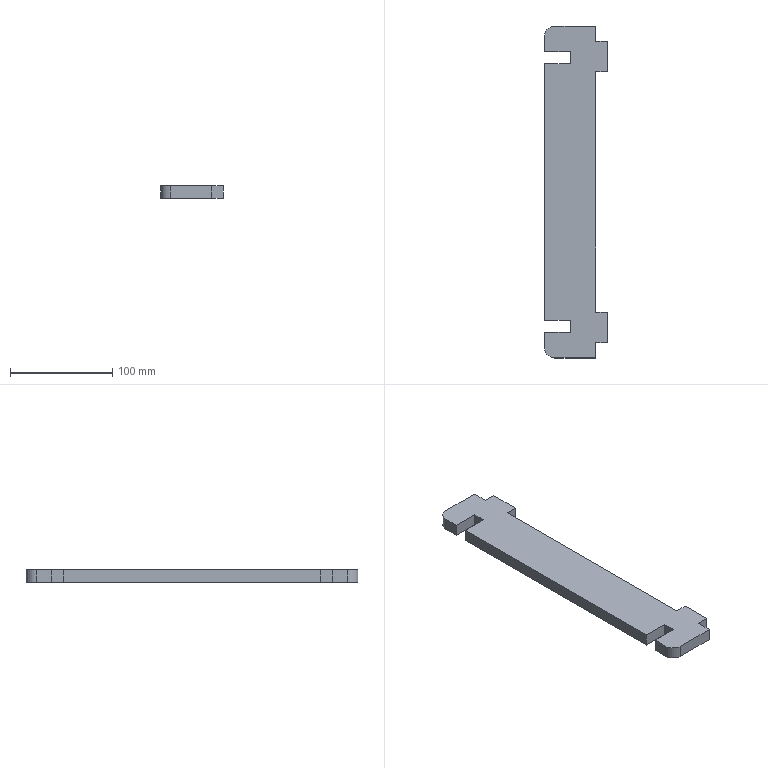Part | SolidWorks | features FlatPattern 1, SMBaseFlange 1, SheetMetal 1 | 1 solid | 24 faces | box 61.5 x 325 x 12 mm | volume 195507 mm3 | plane 22 | cylinder 2 | commonest cylinder face diameters 20 x2
STEP:
#1=CARTESIAN_POINT('',(154.972,127.382,0.));
#2=VERTEX_POINT('',#1);
#3=CARTESIAN_POINT('',(154.972,142.382,0.));
#4=VERTEX_POINT('',#3);
#5=CARTESIAN_POINT('',(154.972,142.382,0.));
#6=DIRECTION('',(0.,1.,0.));
#7=VECTOR('',#6,1000.);
#8=LINE('',#5,#7);
#9=EDGE_CURVE('',#2,#4,#8,.T.);
#10=ORIENTED_EDGE('',*,*,#9,.F.);
#11=CARTESIAN_POINT('',(154.972,127.382,-12.));
#12=VERTEX_POINT('',#11);
#13=CARTESIAN_POINT('',(154.972,127.382,-12.));
#14=DIRECTION('',(0.,0.,1.));
#15=VECTOR('',#14,1000.);
#16=LINE('',#13,#15);
#17=EDGE_CURVE('',#12,#2,#16,.T.);
#18=ORIENTED_EDGE('',*,*,#17,.F.);
#19=CARTESIAN_POINT('',(154.972,142.382,-12.));
#20=VERTEX_POINT('',#19);
#21=CARTESIAN_POINT('',(154.972,142.382,-12.));
#22=DIRECTION('',(0.,1.,0.));
#23=VECTOR('',#22,1000.);
#24=LINE('',#21,#23);
#25=EDGE_CURVE('',#12,#20,#24,.T.);
#26=ORIENTED_EDGE('',*,*,#25,.T.);
#27=CARTESIAN_POINT('',(154.972,142.382,-12.));
#28=DIRECTION('',(0.,0.,1.));
#29=VECTOR('',#28,1000.);
#30=LINE('',#27,#29);
#31=EDGE_CURVE('',#20,#4,#30,.T.);
#32=ORIENTED_EDGE('',*,*,#31,.T.);
#33=EDGE_LOOP('',(#10,#18,#26,#32));
#34=FACE_OUTER_BOUND('',#33,.T.);
#35=CARTESIAN_POINT('',(154.972,142.382,-12.));
#36=DIRECTION('',(1.,0.,0.));
#37=DIRECTION('',(0.,0.,-1.));
#38=AXIS2_PLACEMENT_3D('',#35,#36,#37);
#39=PLANE('',#38);
#40=ADVANCED_FACE('',(#34),#39,.T.);
#41=CARTESIAN_POINT('',(166.472,127.382,0.));
#42=VERTEX_POINT('',#41);
#43=CARTESIAN_POINT('',(154.972,127.382,0.));
#44=DIRECTION('',(-1.,0.,0.));
#45=VECTOR('',#44,1000.);
#46=LINE('',#43,#45);
#47=EDGE_CURVE('',#42,#2,#46,.T.);
#48=ORIENTED_EDGE('',*,*,#47,.F.);
#49=CARTESIAN_POINT('',(166.472,127.382,-12.));
#50=VERTEX_POINT('',#49);
#51=CARTESIAN_POINT('',(166.472,127.382,-12.));
#52=DIRECTION('',(0.,0.,1.));
#53=VECTOR('',#52,1000.);
#54=LINE('',#51,#53);
#55=EDGE_CURVE('',#50,#42,#54,.T.);
#56=ORIENTED_EDGE('',*,*,#55,.F.);
#57=CARTESIAN_POINT('',(154.972,127.382,-12.));
#58=DIRECTION('',(-1.,0.,0.));
#59=VECTOR('',#58,1000.);
#60=LINE('',#57,#59);
#61=EDGE_CURVE('',#50,#12,#60,.T.);
#62=ORIENTED_EDGE('',*,*,#61,.T.);
#63=ORIENTED_EDGE('',*,*,#17,.T.);
#64=EDGE_LOOP('',(#48,#56,#62,#63));
#65=FACE_OUTER_BOUND('',#64,.T.);
#66=CARTESIAN_POINT('',(154.972,127.382,-12.));
#67=DIRECTION('',(0.,1.,0.));
#68=DIRECTION('',(0.,0.,1.));
#69=AXIS2_PLACEMENT_3D('',#66,#67,#68);
#70=PLANE('',#69);
#71=ADVANCED_FACE('',(#65),#70,.T.);
#72=CARTESIAN_POINT('',(166.472,97.382,0.));
#73=VERTEX_POINT('',#72);
#74=CARTESIAN_POINT('',(166.472,127.382,0.));
#75=DIRECTION('',(0.,1.,0.));
#76=VECTOR('',#75,1000.);
#77=LINE('',#74,#76);
#78=EDGE_CURVE('',#73,#42,#77,.T.);
#79=ORIENTED_EDGE('',*,*,#78,.F.);
#80=CARTESIAN_POINT('',(166.472,97.382,-12.));
#81=VERTEX_POINT('',#80);
#82=CARTESIAN_POINT('',(166.472,97.382,-12.));
#83=DIRECTION('',(0.,0.,1.));
#84=VECTOR('',#83,1000.);
#85=LINE('',#82,#84);
#86=EDGE_CURVE('',#81,#73,#85,.T.);
#87=ORIENTED_EDGE('',*,*,#86,.F.);
#88=CARTESIAN_POINT('',(166.472,127.382,-12.));
#89=DIRECTION('',(0.,1.,0.));
#90=VECTOR('',#89,1000.);
#91=LINE('',#88,#90);
#92=EDGE_CURVE('',#81,#50,#91,.T.);
#93=ORIENTED_EDGE('',*,*,#92,.T.);
#94=ORIENTED_EDGE('',*,*,#55,.T.);
#95=EDGE_LOOP('',(#79,#87,#93,#94));
#96=FACE_OUTER_BOUND('',#95,.T.);
#97=CARTESIAN_POINT('',(166.472,127.382,-12.));
#98=DIRECTION('',(1.,0.,0.));
#99=DIRECTION('',(0.,0.,-1.));
#100=AXIS2_PLACEMENT_3D('',#97,#98,#99);
#101=PLANE('',#100);
#102=ADVANCED_FACE('',(#96),#101,.T.);
#103=CARTESIAN_POINT('',(154.972,97.382,0.));
#104=VERTEX_POINT('',#103);
#105=CARTESIAN_POINT('',(166.472,97.382,0.));
#106=DIRECTION('',(1.,0.,0.));
#107=VECTOR('',#106,1000.);
#108=LINE('',#105,#107);
#109=EDGE_CURVE('',#104,#73,#108,.T.);
#110=ORIENTED_EDGE('',*,*,#109,.F.);
#111=CARTESIAN_POINT('',(154.972,97.382,-12.));
#112=VERTEX_POINT('',#111);
#113=CARTESIAN_POINT('',(154.972,97.382,-12.));
#114=DIRECTION('',(0.,0.,1.));
#115=VECTOR('',#114,1000.);
#116=LINE('',#113,#115);
#117=EDGE_CURVE('',#112,#104,#116,.T.);
#118=ORIENTED_EDGE('',*,*,#117,.F.);
#119=CARTESIAN_POINT('',(166.472,97.382,-12.));
#120=DIRECTION('',(1.,0.,0.));
#121=VECTOR('',#120,1000.);
#122=LINE('',#119,#121);
#123=EDGE_CURVE('',#112,#81,#122,.T.);
#124=ORIENTED_EDGE('',*,*,#123,.T.);
#125=ORIENTED_EDGE('',*,*,#86,.T.);
#126=EDGE_LOOP('',(#110,#118,#124,#125));
#127=FACE_OUTER_BOUND('',#126,.T.);
#128=CARTESIAN_POINT('',(166.472,97.382,-12.));
#129=DIRECTION('',(0.,-1.,0.));
#130=DIRECTION('',(0.,0.,-1.));
#131=AXIS2_PLACEMENT_3D('',#128,#129,#130);
#132=PLANE('',#131);
#133=ADVANCED_FACE('',(#127),#132,.T.);
#134=CARTESIAN_POINT('',(154.972,-137.618,0.));
#135=VERTEX_POINT('',#134);
#136=CARTESIAN_POINT('',(154.972,97.382,0.));
#137=DIRECTION('',(0.,1.,0.));
#138=VECTOR('',#137,1000.);
#139=LINE('',#136,#138);
#140=EDGE_CURVE('',#135,#104,#139,.T.);
#141=ORIENTED_EDGE('',*,*,#140,.F.);
#142=CARTESIAN_POINT('',(154.972,-137.618,-12.));
#143=VERTEX_POINT('',#142);
#144=CARTESIAN_POINT('',(154.972,-137.618,-12.));
#145=DIRECTION('',(0.,0.,1.));
#146=VECTOR('',#145,1000.);
#147=LINE('',#144,#146);
#148=EDGE_CURVE('',#143,#135,#147,.T.);
#149=ORIENTED_EDGE('',*,*,#148,.F.);
#150=CARTESIAN_POINT('',(154.972,97.382,-12.));
#151=DIRECTION('',(0.,1.,0.));
#152=VECTOR('',#151,1000.);
#153=LINE('',#150,#152);
#154=EDGE_CURVE('',#143,#112,#153,.T.);
#155=ORIENTED_EDGE('',*,*,#154,.T.);
#156=ORIENTED_EDGE('',*,*,#117,.T.);
#157=EDGE_LOOP('',(#141,#149,#155,#156));
#158=FACE_OUTER_BOUND('',#157,.T.);
#159=CARTESIAN_POINT('',(154.972,97.382,-12.));
#160=DIRECTION('',(1.,0.,0.));
#161=DIRECTION('',(0.,1.,0.));
#162=AXIS2_PLACEMENT_3D('',#159,#160,#161);
#163=PLANE('',#162);
#164=ADVANCED_FACE('',(#158),#163,.T.);
#165=CARTESIAN_POINT('',(166.472,-137.618,0.));
#166=VERTEX_POINT('',#165);
#167=CARTESIAN_POINT('',(154.972,-137.618,0.));
#168=DIRECTION('',(-1.,0.,0.));
#169=VECTOR('',#168,1000.);
#170=LINE('',#167,#169);
#171=EDGE_CURVE('',#166,#135,#170,.T.);
#172=ORIENTED_EDGE('',*,*,#171,.F.);
#173=CARTESIAN_POINT('',(166.472,-137.618,-12.));
#174=VERTEX_POINT('',#173);
#175=CARTESIAN_POINT('',(166.472,-137.618,-12.));
#176=DIRECTION('',(0.,0.,1.));
#177=VECTOR('',#176,1000.);
#178=LINE('',#175,#177);
#179=EDGE_CURVE('',#174,#166,#178,.T.);
#180=ORIENTED_EDGE('',*,*,#179,.F.);
#181=CARTESIAN_POINT('',(154.972,-137.618,-12.));
#182=DIRECTION('',(-1.,0.,0.));
#183=VECTOR('',#182,1000.);
#184=LINE('',#181,#183);
#185=EDGE_CURVE('',#174,#143,#184,.T.);
#186=ORIENTED_EDGE('',*,*,#185,.T.);
#187=ORIENTED_EDGE('',*,*,#148,.T.);
#188=EDGE_LOOP('',(#172,#180,#186,#187));
#189=FACE_OUTER_BOUND('',#188,.T.);
#190=CARTESIAN_POINT('',(154.972,-137.618,-12.));
#191=DIRECTION('',(0.,1.,0.));
#192=DIRECTION('',(0.,0.,1.));
#193=AXIS2_PLACEMENT_3D('',#190,#191,#192);
#194=PLANE('',#193);
#195=ADVANCED_FACE('',(#189),#194,.T.);
#196=CARTESIAN_POINT('',(166.472,-167.618,0.));
#197=VERTEX_POINT('',#196);
#198=CARTESIAN_POINT('',(166.472,-137.618,0.));
#199=DIRECTION('',(0.,1.,0.));
#200=VECTOR('',#199,1000.);
#201=LINE('',#198,#200);
#202=EDGE_CURVE('',#197,#166,#201,.T.);
#203=ORIENTED_EDGE('',*,*,#202,.F.);
#204=CARTESIAN_POINT('',(166.472,-167.618,-12.));
#205=VERTEX_POINT('',#204);
#206=CARTESIAN_POINT('',(166.472,-167.618,-12.));
#207=DIRECTION('',(0.,0.,1.));
#208=VECTOR('',#207,1000.);
#209=LINE('',#206,#208);
#210=EDGE_CURVE('',#205,#197,#209,.T.);
#211=ORIENTED_EDGE('',*,*,#210,.F.);
#212=CARTESIAN_POINT('',(166.472,-137.618,-12.));
#213=DIRECTION('',(0.,1.,0.));
#214=VECTOR('',#213,1000.);
#215=LINE('',#212,#214);
#216=EDGE_CURVE('',#205,#174,#215,.T.);
#217=ORIENTED_EDGE('',*,*,#216,.T.);
#218=ORIENTED_EDGE('',*,*,#179,.T.);
#219=EDGE_LOOP('',(#203,#211,#217,#218));
#220=FACE_OUTER_BOUND('',#219,.T.);
#221=CARTESIAN_POINT('',(166.472,-137.618,-12.));
#222=DIRECTION('',(1.,0.,0.));
#223=DIRECTION('',(0.,0.,-1.));
#224=AXIS2_PLACEMENT_3D('',#221,#222,#223);
#225=PLANE('',#224);
#226=ADVANCED_FACE('',(#220),#225,.T.);
#227=CARTESIAN_POINT('',(154.972,-167.618,0.));
#228=VERTEX_POINT('',#227);
#229=CARTESIAN_POINT('',(166.472,-167.618,0.));
#230=DIRECTION('',(1.,0.,0.));
#231=VECTOR('',#230,1000.);
#232=LINE('',#229,#231);
#233=EDGE_CURVE('',#228,#197,#232,.T.);
#234=ORIENTED_EDGE('',*,*,#233,.F.);
#235=CARTESIAN_POINT('',(154.972,-167.618,-12.));
#236=VERTEX_POINT('',#235);
#237=CARTESIAN_POINT('',(154.972,-167.618,-12.));
#238=DIRECTION('',(0.,0.,1.));
#239=VECTOR('',#238,1000.);
#240=LINE('',#237,#239);
#241=EDGE_CURVE('',#236,#228,#240,.T.);
#242=ORIENTED_EDGE('',*,*,#241,.F.);
#243=CARTESIAN_POINT('',(166.472,-167.618,-12.));
#244=DIRECTION('',(1.,0.,0.));
#245=VECTOR('',#244,1000.);
#246=LINE('',#243,#245);
#247=EDGE_CURVE('',#236,#205,#246,.T.);
#248=ORIENTED_EDGE('',*,*,#247,.T.);
#249=ORIENTED_EDGE('',*,*,#210,.T.);
#250=EDGE_LOOP('',(#234,#242,#248,#249));
#251=FACE_OUTER_BOUND('',#250,.T.);
#252=CARTESIAN_POINT('',(166.472,-167.618,-12.));
#253=DIRECTION('',(0.,-1.,0.));
#254=DIRECTION('',(0.,0.,-1.));
#255=AXIS2_PLACEMENT_3D('',#252,#253,#254);
#256=PLANE('',#255);
#257=ADVANCED_FACE('',(#251),#256,.T.);
#258=CARTESIAN_POINT('',(154.972,-182.618,0.));
#259=VERTEX_POINT('',#258);
#260=CARTESIAN_POINT('',(154.972,-167.618,0.));
#261=DIRECTION('',(0.,1.,0.));
#262=VECTOR('',#261,1000.);
#263=LINE('',#260,#262);
#264=EDGE_CURVE('',#259,#228,#263,.T.);
#265=ORIENTED_EDGE('',*,*,#264,.F.);
#266=CARTESIAN_POINT('',(154.972,-182.618,-12.));
#267=VERTEX_POINT('',#266);
#268=CARTESIAN_POINT('',(154.972,-182.618,-12.));
#269=DIRECTION('',(0.,0.,1.));
#270=VECTOR('',#269,1000.);
#271=LINE('',#268,#270);
#272=EDGE_CURVE('',#267,#259,#271,.T.);
#273=ORIENTED_EDGE('',*,*,#272,.F.);
#274=CARTESIAN_POINT('',(154.972,-167.618,-12.));
#275=DIRECTION('',(0.,1.,0.));
#276=VECTOR('',#275,1000.);
#277=LINE('',#274,#276);
#278=EDGE_CURVE('',#267,#236,#277,.T.);
#279=ORIENTED_EDGE('',*,*,#278,.T.);
#280=ORIENTED_EDGE('',*,*,#241,.T.);
#281=EDGE_LOOP('',(#265,#273,#279,#280));
#282=FACE_OUTER_BOUND('',#281,.T.);
#283=CARTESIAN_POINT('',(154.972,-167.618,-12.));
#284=DIRECTION('',(1.,0.,0.));
#285=DIRECTION('',(0.,1.,0.));
#286=AXIS2_PLACEMENT_3D('',#283,#284,#285);
#287=PLANE('',#286);
#288=ADVANCED_FACE('',(#282),#287,.T.);
#289=CARTESIAN_POINT('',(114.972,-182.618,0.));
#290=VERTEX_POINT('',#289);
#291=CARTESIAN_POINT('',(154.972,-182.618,0.));
#292=DIRECTION('',(1.,0.,0.));
#293=VECTOR('',#292,1000.);
#294=LINE('',#291,#293);
#295=EDGE_CURVE('',#290,#259,#294,.T.);
#296=ORIENTED_EDGE('',*,*,#295,.F.);
#297=CARTESIAN_POINT('',(114.972,-182.618,-12.));
#298=VERTEX_POINT('',#297);
#299=CARTESIAN_POINT('',(114.972,-182.618,-12.));
#300=DIRECTION('',(0.,0.,1.));
#301=VECTOR('',#300,1000.);
#302=LINE('',#299,#301);
#303=EDGE_CURVE('',#298,#290,#302,.T.);
#304=ORIENTED_EDGE('',*,*,#303,.F.);
#305=CARTESIAN_POINT('',(154.972,-182.618,-12.));
#306=DIRECTION('',(1.,0.,0.));
#307=VECTOR('',#306,1000.);
#308=LINE('',#305,#307);
#309=EDGE_CURVE('',#298,#267,#308,.T.);
#310=ORIENTED_EDGE('',*,*,#309,.T.);
#311=ORIENTED_EDGE('',*,*,#272,.T.);
#312=EDGE_LOOP('',(#296,#304,#310,#311));
#313=FACE_OUTER_BOUND('',#312,.T.);
#314=CARTESIAN_POINT('',(154.972,-182.618,-12.));
#315=DIRECTION('',(0.,-1.,0.));
#316=DIRECTION('',(1.,0.,0.));
#317=AXIS2_PLACEMENT_3D('',#314,#315,#316);
#318=PLANE('',#317);
#319=ADVANCED_FACE('',(#313),#318,.T.);
#320=CARTESIAN_POINT('',(104.972,-172.618,0.));
#321=VERTEX_POINT('',#320);
#322=CARTESIAN_POINT('',(114.972,-172.618,0.));
#323=DIRECTION('',(0.,0.,1.));
#324=DIRECTION('',(-1.,0.,0.));
#325=AXIS2_PLACEMENT_3D('',#322,#323,#324);
#326=CIRCLE('',#325,10.);
#327=EDGE_CURVE('',#321,#290,#326,.T.);
#328=ORIENTED_EDGE('',*,*,#327,.F.);
#329=CARTESIAN_POINT('',(104.972,-172.618,-12.));
#330=VERTEX_POINT('',#329);
#331=CARTESIAN_POINT('',(104.972,-172.618,-12.));
#332=DIRECTION('',(0.,0.,1.));
#333=VECTOR('',#332,1000.);
#334=LINE('',#331,#333);
#335=EDGE_CURVE('',#330,#321,#334,.T.);
#336=ORIENTED_EDGE('',*,*,#335,.F.);
#337=CARTESIAN_POINT('',(114.972,-172.618,-12.));
#338=DIRECTION('',(0.,0.,1.));
#339=DIRECTION('',(-1.,0.,0.));
#340=AXIS2_PLACEMENT_3D('',#337,#338,#339);
#341=CIRCLE('',#340,10.);
#342=EDGE_CURVE('',#330,#298,#341,.T.);
#343=ORIENTED_EDGE('',*,*,#342,.T.);
#344=ORIENTED_EDGE('',*,*,#303,.T.);
#345=EDGE_LOOP('',(#328,#336,#343,#344));
#346=FACE_OUTER_BOUND('',#345,.T.);
#347=CARTESIAN_POINT('',(114.972,-172.618,-12.));
#348=DIRECTION('',(0.,0.,1.));
#349=DIRECTION('',(1.,0.,0.));
#350=AXIS2_PLACEMENT_3D('',#347,#348,#349);
#351=CYLINDRICAL_SURFACE('',#350,10.);
#352=ADVANCED_FACE('',(#346),#351,.T.);
#353=CARTESIAN_POINT('',(104.972,-157.618,0.));
#354=VERTEX_POINT('',#353);
#355=CARTESIAN_POINT('',(104.972,-157.618,0.));
#356=DIRECTION('',(0.,-1.,0.));
#357=VECTOR('',#356,1000.);
#358=LINE('',#355,#357);
#359=EDGE_CURVE('',#354,#321,#358,.T.);
#360=ORIENTED_EDGE('',*,*,#359,.F.);
#361=CARTESIAN_POINT('',(104.972,-157.618,-12.));
#362=VERTEX_POINT('',#361);
#363=CARTESIAN_POINT('',(104.972,-157.618,-12.));
#364=DIRECTION('',(0.,0.,1.));
#365=VECTOR('',#364,1000.);
#366=LINE('',#363,#365);
#367=EDGE_CURVE('',#362,#354,#366,.T.);
#368=ORIENTED_EDGE('',*,*,#367,.F.);
#369=CARTESIAN_POINT('',(104.972,-157.618,-12.));
#370=DIRECTION('',(0.,-1.,0.));
#371=VECTOR('',#370,1000.);
#372=LINE('',#369,#371);
#373=EDGE_CURVE('',#362,#330,#372,.T.);
#374=ORIENTED_EDGE('',*,*,#373,.T.);
#375=ORIENTED_EDGE('',*,*,#335,.T.);
#376=EDGE_LOOP('',(#360,#368,#374,#375));
#377=FACE_OUTER_BOUND('',#376,.T.);
#378=CARTESIAN_POINT('',(104.972,-157.618,-12.));
#379=DIRECTION('',(-1.,0.,0.));
#380=DIRECTION('',(0.,0.,1.));
#381=AXIS2_PLACEMENT_3D('',#378,#379,#380);
#382=PLANE('',#381);
#383=ADVANCED_FACE('',(#377),#382,.T.);
#384=CARTESIAN_POINT('',(130.172,-157.618,0.));
#385=VERTEX_POINT('',#384);
#386=CARTESIAN_POINT('',(104.972,-157.618,0.));
#387=DIRECTION('',(-1.,0.,0.));
#388=VECTOR('',#387,1000.);
#389=LINE('',#386,#388);
#390=EDGE_CURVE('',#385,#354,#389,.T.);
#391=ORIENTED_EDGE('',*,*,#390,.F.);
#392=CARTESIAN_POINT('',(130.172,-157.618,-12.));
#393=VERTEX_POINT('',#392);
#394=CARTESIAN_POINT('',(130.172,-157.618,-12.));
#395=DIRECTION('',(0.,0.,1.));
#396=VECTOR('',#395,1000.);
#397=LINE('',#394,#396);
#398=EDGE_CURVE('',#393,#385,#397,.T.);
#399=ORIENTED_EDGE('',*,*,#398,.F.);
#400=CARTESIAN_POINT('',(104.972,-157.618,-12.));
#401=DIRECTION('',(-1.,0.,0.));
#402=VECTOR('',#401,1000.);
#403=LINE('',#400,#402);
#404=EDGE_CURVE('',#393,#362,#403,.T.);
#405=ORIENTED_EDGE('',*,*,#404,.T.);
#406=ORIENTED_EDGE('',*,*,#367,.T.);
#407=EDGE_LOOP('',(#391,#399,#405,#406));
#408=FACE_OUTER_BOUND('',#407,.T.);
#409=CARTESIAN_POINT('',(104.972,-157.618,-12.));
#410=DIRECTION('',(0.,1.,0.));
#411=DIRECTION('',(-1.,0.,0.));
#412=AXIS2_PLACEMENT_3D('',#409,#410,#411);
#413=PLANE('',#412);
#414=ADVANCED_FACE('',(#408),#413,.T.);
#415=CARTESIAN_POINT('',(130.172,-145.618,0.));
#416=VERTEX_POINT('',#415);
#417=CARTESIAN_POINT('',(130.172,-157.618,0.));
#418=DIRECTION('',(0.,-1.,0.));
#419=VECTOR('',#418,1000.);
#420=LINE('',#417,#419);
#421=EDGE_CURVE('',#416,#385,#420,.T.);
#422=ORIENTED_EDGE('',*,*,#421,.F.);
#423=CARTESIAN_POINT('',(130.172,-145.618,-12.));
#424=VERTEX_POINT('',#423);
#425=CARTESIAN_POINT('',(130.172,-145.618,-12.));
#426=DIRECTION('',(0.,0.,1.));
#427=VECTOR('',#426,1000.);
#428=LINE('',#425,#427);
#429=EDGE_CURVE('',#424,#416,#428,.T.);
#430=ORIENTED_EDGE('',*,*,#429,.F.);
#431=CARTESIAN_POINT('',(130.172,-157.618,-12.));
#432=DIRECTION('',(0.,-1.,0.));
#433=VECTOR('',#432,1000.);
#434=LINE('',#431,#433);
#435=EDGE_CURVE('',#424,#393,#434,.T.);
#436=ORIENTED_EDGE('',*,*,#435,.T.);
#437=ORIENTED_EDGE('',*,*,#398,.T.);
#438=EDGE_LOOP('',(#422,#430,#436,#437));
#439=FACE_OUTER_BOUND('',#438,.T.);
#440=CARTESIAN_POINT('',(130.172,-157.618,-12.));
#441=DIRECTION('',(-1.,0.,0.));
#442=DIRECTION('',(0.,0.,1.));
#443=AXIS2_PLACEMENT_3D('',#440,#441,#442);
#444=PLANE('',#443);
#445=ADVANCED_FACE('',(#439),#444,.T.);
#446=CARTESIAN_POINT('',(104.972,-145.618,0.));
#447=VERTEX_POINT('',#446);
#448=CARTESIAN_POINT('',(130.172,-145.618,0.));
#449=DIRECTION('',(1.,0.,0.));
#450=VECTOR('',#449,1000.);
#451=LINE('',#448,#450);
#452=EDGE_CURVE('',#447,#416,#451,.T.);
#453=ORIENTED_EDGE('',*,*,#452,.F.);
#454=CARTESIAN_POINT('',(104.972,-145.618,-12.));
#455=VERTEX_POINT('',#454);
#456=CARTESIAN_POINT('',(104.972,-145.618,-12.));
#457=DIRECTION('',(0.,0.,1.));
#458=VECTOR('',#457,1000.);
#459=LINE('',#456,#458);
#460=EDGE_CURVE('',#455,#447,#459,.T.);
#461=ORIENTED_EDGE('',*,*,#460,.F.);
#462=CARTESIAN_POINT('',(130.172,-145.618,-12.));
#463=DIRECTION('',(1.,0.,0.));
#464=VECTOR('',#463,1000.);
#465=LINE('',#462,#464);
#466=EDGE_CURVE('',#455,#424,#465,.T.);
#467=ORIENTED_EDGE('',*,*,#466,.T.);
#468=ORIENTED_EDGE('',*,*,#429,.T.);
#469=EDGE_LOOP('',(#453,#461,#467,#468));
#470=FACE_OUTER_BOUND('',#469,.T.);
#471=CARTESIAN_POINT('',(130.172,-145.618,-12.));
#472=DIRECTION('',(0.,-1.,0.));
#473=DIRECTION('',(1.,0.,0.));
#474=AXIS2_PLACEMENT_3D('',#471,#472,#473);
#475=PLANE('',#474);
#476=ADVANCED_FACE('',(#470),#475,.T.);
#477=CARTESIAN_POINT('',(104.972,105.382,0.));
#478=VERTEX_POINT('',#477);
#479=CARTESIAN_POINT('',(104.972,105.382,0.));
#480=DIRECTION('',(0.,-1.,0.));
#481=VECTOR('',#480,1000.);
#482=LINE('',#479,#481);
#483=EDGE_CURVE('',#478,#447,#482,.T.);
#484=ORIENTED_EDGE('',*,*,#483,.F.);
#485=CARTESIAN_POINT('',(104.972,105.382,-12.));
#486=VERTEX_POINT('',#485);
#487=CARTESIAN_POINT('',(104.972,105.382,-12.));
#488=DIRECTION('',(0.,0.,1.));
#489=VECTOR('',#488,1000.);
#490=LINE('',#487,#489);
#491=EDGE_CURVE('',#486,#478,#490,.T.);
#492=ORIENTED_EDGE('',*,*,#491,.F.);
#493=CARTESIAN_POINT('',(104.972,105.382,-12.));
#494=DIRECTION('',(0.,-1.,0.));
#495=VECTOR('',#494,1000.);
#496=LINE('',#493,#495);
#497=EDGE_CURVE('',#486,#455,#496,.T.);
#498=ORIENTED_EDGE('',*,*,#497,.T.);
#499=ORIENTED_EDGE('',*,*,#460,.T.);
#500=EDGE_LOOP('',(#484,#492,#498,#499));
#501=FACE_OUTER_BOUND('',#500,.T.);
#502=CARTESIAN_POINT('',(104.972,105.382,-12.));
#503=DIRECTION('',(-1.,0.,0.));
#504=DIRECTION('',(0.,-1.,0.));
#505=AXIS2_PLACEMENT_3D('',#502,#503,#504);
#506=PLANE('',#505);
#507=ADVANCED_FACE('',(#501),#506,.T.);
#508=CARTESIAN_POINT('',(130.172,105.382,0.));
#509=VERTEX_POINT('',#508);
#510=CARTESIAN_POINT('',(104.972,105.382,0.));
#511=DIRECTION('',(-1.,0.,0.));
#512=VECTOR('',#511,1000.);
#513=LINE('',#510,#512);
#514=EDGE_CURVE('',#509,#478,#513,.T.);
#515=ORIENTED_EDGE('',*,*,#514,.F.);
#516=CARTESIAN_POINT('',(130.172,105.382,-12.));
#517=VERTEX_POINT('',#516);
#518=CARTESIAN_POINT('',(130.172,105.382,-12.));
#519=DIRECTION('',(0.,0.,1.));
#520=VECTOR('',#519,1000.);
#521=LINE('',#518,#520);
#522=EDGE_CURVE('',#517,#509,#521,.T.);
#523=ORIENTED_EDGE('',*,*,#522,.F.);
#524=CARTESIAN_POINT('',(104.972,105.382,-12.));
#525=DIRECTION('',(-1.,0.,0.));
#526=VECTOR('',#525,1000.);
#527=LINE('',#524,#526);
#528=EDGE_CURVE('',#517,#486,#527,.T.);
#529=ORIENTED_EDGE('',*,*,#528,.T.);
#530=ORIENTED_EDGE('',*,*,#491,.T.);
#531=EDGE_LOOP('',(#515,#523,#529,#530));
#532=FACE_OUTER_BOUND('',#531,.T.);
#533=CARTESIAN_POINT('',(104.972,105.382,-12.));
#534=DIRECTION('',(0.,1.,0.));
#535=DIRECTION('',(-1.,0.,0.));
#536=AXIS2_PLACEMENT_3D('',#533,#534,#535);
#537=PLANE('',#536);
#538=ADVANCED_FACE('',(#532),#537,.T.);
#539=CARTESIAN_POINT('',(130.172,117.382,0.));
#540=VERTEX_POINT('',#539);
#541=CARTESIAN_POINT('',(130.172,105.382,0.));
#542=DIRECTION('',(0.,-1.,0.));
#543=VECTOR('',#542,1000.);
#544=LINE('',#541,#543);
#545=EDGE_CURVE('',#540,#509,#544,.T.);
#546=ORIENTED_EDGE('',*,*,#545,.F.);
#547=CARTESIAN_POINT('',(130.172,117.382,-12.));
#548=VERTEX_POINT('',#547);
#549=CARTESIAN_POINT('',(130.172,117.382,-12.));
#550=DIRECTION('',(0.,0.,1.));
#551=VECTOR('',#550,1000.);
#552=LINE('',#549,#551);
#553=EDGE_CURVE('',#548,#540,#552,.T.);
#554=ORIENTED_EDGE('',*,*,#553,.F.);
#555=CARTESIAN_POINT('',(130.172,105.382,-12.));
#556=DIRECTION('',(0.,-1.,0.));
#557=VECTOR('',#556,1000.);
#558=LINE('',#555,#557);
#559=EDGE_CURVE('',#548,#517,#558,.T.);
#560=ORIENTED_EDGE('',*,*,#559,.T.);
#561=ORIENTED_EDGE('',*,*,#522,.T.);
#562=EDGE_LOOP('',(#546,#554,#560,#561));
#563=FACE_OUTER_BOUND('',#562,.T.);
#564=CARTESIAN_POINT('',(130.172,105.382,-12.));
#565=DIRECTION('',(-1.,0.,0.));
#566=DIRECTION('',(0.,0.,1.));
#567=AXIS2_PLACEMENT_3D('',#564,#565,#566);
#568=PLANE('',#567);
#569=ADVANCED_FACE('',(#563),#568,.T.);
#570=CARTESIAN_POINT('',(104.972,117.382,0.));
#571=VERTEX_POINT('',#570);
#572=CARTESIAN_POINT('',(130.172,117.382,0.));
#573=DIRECTION('',(1.,0.,0.));
#574=VECTOR('',#573,1000.);
#575=LINE('',#572,#574);
#576=EDGE_CURVE('',#571,#540,#575,.T.);
#577=ORIENTED_EDGE('',*,*,#576,.F.);
#578=CARTESIAN_POINT('',(104.972,117.382,-12.));
#579=VERTEX_POINT('',#578);
#580=CARTESIAN_POINT('',(104.972,117.382,-12.));
#581=DIRECTION('',(0.,0.,1.));
#582=VECTOR('',#581,1000.);
#583=LINE('',#580,#582);
#584=EDGE_CURVE('',#579,#571,#583,.T.);
#585=ORIENTED_EDGE('',*,*,#584,.F.);
#586=CARTESIAN_POINT('',(130.172,117.382,-12.));
#587=DIRECTION('',(1.,0.,0.));
#588=VECTOR('',#587,1000.);
#589=LINE('',#586,#588);
#590=EDGE_CURVE('',#579,#548,#589,.T.);
#591=ORIENTED_EDGE('',*,*,#590,.T.);
#592=ORIENTED_EDGE('',*,*,#553,.T.);
#593=EDGE_LOOP('',(#577,#585,#591,#592));
#594=FACE_OUTER_BOUND('',#593,.T.);
#595=CARTESIAN_POINT('',(130.172,117.382,-12.));
#596=DIRECTION('',(0.,-1.,0.));
#597=DIRECTION('',(0.,0.,-1.));
#598=AXIS2_PLACEMENT_3D('',#595,#596,#597);
#599=PLANE('',#598);
#600=ADVANCED_FACE('',(#594),#599,.T.);
#601=CARTESIAN_POINT('',(104.972,132.382,0.));
#602=VERTEX_POINT('',#601);
#603=CARTESIAN_POINT('',(104.972,132.382,0.));
#604=DIRECTION('',(0.,-1.,0.));
#605=VECTOR('',#604,1000.);
#606=LINE('',#603,#605);
#607=EDGE_CURVE('',#602,#571,#606,.T.);
#608=ORIENTED_EDGE('',*,*,#607,.F.);
#609=CARTESIAN_POINT('',(104.972,132.382,-12.));
#610=VERTEX_POINT('',#609);
#611=CARTESIAN_POINT('',(104.972,132.382,-12.));
#612=DIRECTION('',(0.,0.,1.));
#613=VECTOR('',#612,1000.);
#614=LINE('',#611,#613);
#615=EDGE_CURVE('',#610,#602,#614,.T.);
#616=ORIENTED_EDGE('',*,*,#615,.F.);
#617=CARTESIAN_POINT('',(104.972,132.382,-12.));
#618=DIRECTION('',(0.,-1.,0.));
#619=VECTOR('',#618,1000.);
#620=LINE('',#617,#619);
#621=EDGE_CURVE('',#610,#579,#620,.T.);
#622=ORIENTED_EDGE('',*,*,#621,.T.);
#623=ORIENTED_EDGE('',*,*,#584,.T.);
#624=EDGE_LOOP('',(#608,#616,#622,#623));
#625=FACE_OUTER_BOUND('',#624,.T.);
#626=CARTESIAN_POINT('',(104.972,132.382,-12.));
#627=DIRECTION('',(-1.,0.,0.));
#628=DIRECTION('',(0.,0.,1.));
#629=AXIS2_PLACEMENT_3D('',#626,#627,#628);
#630=PLANE('',#629);
#631=ADVANCED_FACE('',(#625),#630,.T.);
#632=CARTESIAN_POINT('',(114.972,142.382,0.));
#633=VERTEX_POINT('',#632);
#634=CARTESIAN_POINT('',(114.972,132.382,0.));
#635=DIRECTION('',(0.,0.,1.));
#636=DIRECTION('',(1.,0.,0.));
#637=AXIS2_PLACEMENT_3D('',#634,#635,#636);
#638=CIRCLE('',#637,10.);
#639=EDGE_CURVE('',#633,#602,#638,.T.);
#640=ORIENTED_EDGE('',*,*,#639,.F.);
#641=CARTESIAN_POINT('',(114.972,142.382,-12.));
#642=VERTEX_POINT('',#641);
#643=CARTESIAN_POINT('',(114.972,142.382,-12.));
#644=DIRECTION('',(0.,0.,1.));
#645=VECTOR('',#644,1000.);
#646=LINE('',#643,#645);
#647=EDGE_CURVE('',#642,#633,#646,.T.);
#648=ORIENTED_EDGE('',*,*,#647,.F.);
#649=CARTESIAN_POINT('',(114.972,132.382,-12.));
#650=DIRECTION('',(0.,0.,1.));
#651=DIRECTION('',(1.,0.,0.));
#652=AXIS2_PLACEMENT_3D('',#649,#650,#651);
#653=CIRCLE('',#652,10.);
#654=EDGE_CURVE('',#642,#610,#653,.T.);
#655=ORIENTED_EDGE('',*,*,#654,.T.);
#656=ORIENTED_EDGE('',*,*,#615,.T.);
#657=EDGE_LOOP('',(#640,#648,#655,#656));
#658=FACE_OUTER_BOUND('',#657,.T.);
#659=CARTESIAN_POINT('',(114.972,132.382,-12.));
#660=DIRECTION('',(0.,0.,1.));
#661=DIRECTION('',(1.,0.,0.));
#662=AXIS2_PLACEMENT_3D('',#659,#660,#661);
#663=CYLINDRICAL_SURFACE('',#662,10.);
#664=ADVANCED_FACE('',(#658),#663,.T.);
#665=CARTESIAN_POINT('',(154.972,142.382,0.));
#666=DIRECTION('',(-1.,0.,0.));
#667=VECTOR('',#666,1000.);
#668=LINE('',#665,#667);
#669=EDGE_CURVE('',#4,#633,#668,.T.);
#670=ORIENTED_EDGE('',*,*,#669,.F.);
#671=ORIENTED_EDGE('',*,*,#31,.F.);
#672=CARTESIAN_POINT('',(154.972,142.382,-12.));
#673=DIRECTION('',(-1.,0.,0.));
#674=VECTOR('',#673,1000.);
#675=LINE('',#672,#674);
#676=EDGE_CURVE('',#20,#642,#675,.T.);
#677=ORIENTED_EDGE('',*,*,#676,.T.);
#678=ORIENTED_EDGE('',*,*,#647,.T.);
#679=EDGE_LOOP('',(#670,#671,#677,#678));
#680=FACE_OUTER_BOUND('',#679,.T.);
#681=CARTESIAN_POINT('',(154.972,142.382,-12.));
#682=DIRECTION('',(0.,1.,0.));
#683=DIRECTION('',(0.,0.,1.));
#684=AXIS2_PLACEMENT_3D('',#681,#682,#683);
#685=PLANE('',#684);
#686=ADVANCED_FACE('',(#680),#685,.T.);
#687=ORIENTED_EDGE('',*,*,#25,.F.);
#688=ORIENTED_EDGE('',*,*,#61,.F.);
#689=ORIENTED_EDGE('',*,*,#92,.F.);
#690=ORIENTED_EDGE('',*,*,#123,.F.);
#691=ORIENTED_EDGE('',*,*,#154,.F.);
#692=ORIENTED_EDGE('',*,*,#185,.F.);
#693=ORIENTED_EDGE('',*,*,#216,.F.);
#694=ORIENTED_EDGE('',*,*,#247,.F.);
#695=ORIENTED_EDGE('',*,*,#278,.F.);
#696=ORIENTED_EDGE('',*,*,#309,.F.);
#697=ORIENTED_EDGE('',*,*,#342,.F.);
#698=ORIENTED_EDGE('',*,*,#373,.F.);
#699=ORIENTED_EDGE('',*,*,#404,.F.);
#700=ORIENTED_EDGE('',*,*,#435,.F.);
#701=ORIENTED_EDGE('',*,*,#466,.F.);
#702=ORIENTED_EDGE('',*,*,#497,.F.);
#703=ORIENTED_EDGE('',*,*,#528,.F.);
#704=ORIENTED_EDGE('',*,*,#559,.F.);
#705=ORIENTED_EDGE('',*,*,#590,.F.);
#706=ORIENTED_EDGE('',*,*,#621,.F.);
#707=ORIENTED_EDGE('',*,*,#654,.F.);
#708=ORIENTED_EDGE('',*,*,#676,.F.);
#709=EDGE_LOOP('',(#687,#688,#689,#690,#691,#692,#693,#694,#695,#696,#697,#698,#699,#700,#701,#702,#703,#704,#705,#706,#707,#708));
#710=FACE_OUTER_BOUND('',#709,.T.);
#711=CARTESIAN_POINT('',(114.972,-172.618,-12.));
#712=DIRECTION('',(0.,0.,-1.));
#713=DIRECTION('',(-1.,0.,0.));
#714=AXIS2_PLACEMENT_3D('',#711,#712,#713);
#715=PLANE('',#714);
#716=ADVANCED_FACE('',(#710),#715,.T.);
#717=ORIENTED_EDGE('',*,*,#9,.T.);
#718=ORIENTED_EDGE('',*,*,#669,.T.);
#719=ORIENTED_EDGE('',*,*,#639,.T.);
#720=ORIENTED_EDGE('',*,*,#607,.T.);
#721=ORIENTED_EDGE('',*,*,#576,.T.);
#722=ORIENTED_EDGE('',*,*,#545,.T.);
#723=ORIENTED_EDGE('',*,*,#514,.T.);
#724=ORIENTED_EDGE('',*,*,#483,.T.);
#725=ORIENTED_EDGE('',*,*,#452,.T.);
#726=ORIENTED_EDGE('',*,*,#421,.T.);
#727=ORIENTED_EDGE('',*,*,#390,.T.);
#728=ORIENTED_EDGE('',*,*,#359,.T.);
#729=ORIENTED_EDGE('',*,*,#327,.T.);
#730=ORIENTED_EDGE('',*,*,#295,.T.);
#731=ORIENTED_EDGE('',*,*,#264,.T.);
#732=ORIENTED_EDGE('',*,*,#233,.T.);
#733=ORIENTED_EDGE('',*,*,#202,.T.);
#734=ORIENTED_EDGE('',*,*,#171,.T.);
#735=ORIENTED_EDGE('',*,*,#140,.T.);
#736=ORIENTED_EDGE('',*,*,#109,.T.);
#737=ORIENTED_EDGE('',*,*,#78,.T.);
#738=ORIENTED_EDGE('',*,*,#47,.T.);
#739=EDGE_LOOP('',(#717,#718,#719,#720,#721,#722,#723,#724,#725,#726,#727,#728,#729,#730,#731,#732,#733,#734,#735,#736,#737,#738));
#740=FACE_OUTER_BOUND('',#739,.T.);
#741=CARTESIAN_POINT('',(114.972,-172.618,0.));
#742=DIRECTION('',(0.,0.,-1.));
#743=DIRECTION('',(-1.,0.,0.));
#744=AXIS2_PLACEMENT_3D('',#741,#742,#743);
#745=PLANE('',#744);
#746=ADVANCED_FACE('',(#740),#745,.F.);
#747=CLOSED_SHELL('',(#40,#71,#102,#133,#164,#195,#226,#257,#288,#319,#352,#383,#414,#445,#476,#507,#538,#569,#600,#631,#664,#686,#716,#746));
#748=MANIFOLD_SOLID_BREP('',#747);
#749=CARTESIAN_POINT('',(0.,0.,0.));
#750=DIRECTION('',(0.,0.,1.));
#751=DIRECTION('',(1.,0.,0.));
#752=AXIS2_PLACEMENT_3D('',#749,#750,#751);
#753=(LENGTH_UNIT()NAMED_UNIT(*)SI_UNIT(.MILLI.,.METRE.));
#754=UNCERTAINTY_MEASURE_WITH_UNIT(LENGTH_MEASURE(0.00001),#753,'','');
#755=(NAMED_UNIT(*)PLANE_ANGLE_UNIT()SI_UNIT($,.RADIAN.));
#756=(NAMED_UNIT(*)SI_UNIT($,.STERADIAN.)SOLID_ANGLE_UNIT());
#757=(GEOMETRIC_REPRESENTATION_CONTEXT(3)GLOBAL_UNCERTAINTY_ASSIGNED_CONTEXT((#754))GLOBAL_UNIT_ASSIGNED_CONTEXT((#753,#755,#756))REPRESENTATION_CONTEXT('',''));
#758=ADVANCED_BREP_SHAPE_REPRESENTATION('',(#748,#752),#757);